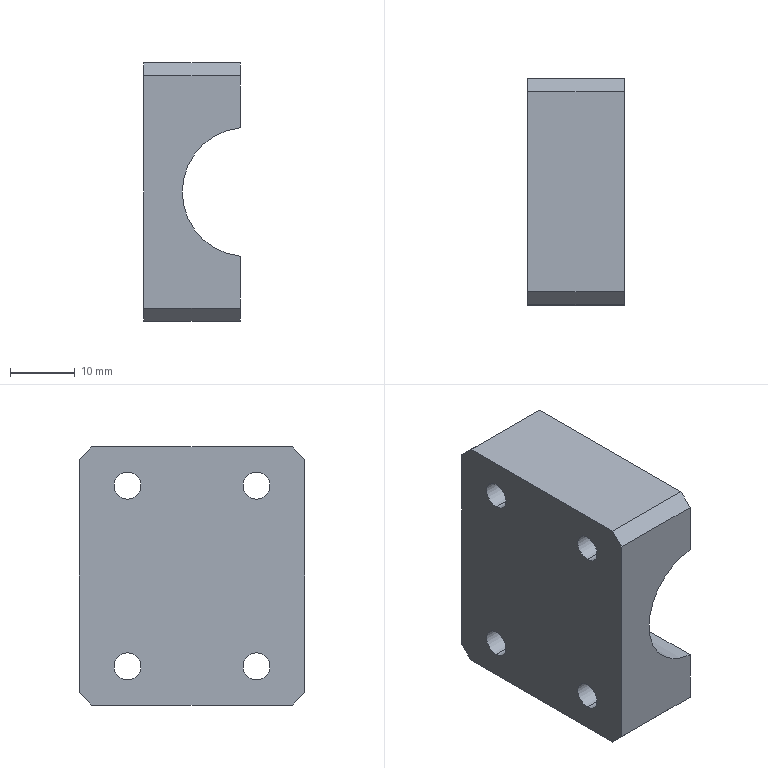Part | SolidWorks | features Chamfer 1, Extrusion 1, HoleWzd 1 | 1 solid | 20 faces | box 15 x 35 x 40 mm | volume 15250 mm3 | plane 11 | cylinder 9 | commonest cylinder face diameters 4.2 x8 20 x1
STEP:
#1=CARTESIAN_POINT('',(-7.5,10.,16.1));
#2=VERTEX_POINT('',#1);
#3=CARTESIAN_POINT('',(-7.5,10.,11.9));
#4=VERTEX_POINT('',#3);
#5=CARTESIAN_POINT('',(-7.5,10.,14.));
#6=DIRECTION('',(1.,0.,0.));
#7=DIRECTION('',(0.,0.,-1.));
#8=AXIS2_PLACEMENT_3D('',#5,#6,#7);
#9=CIRCLE('',#8,2.1);
#10=EDGE_CURVE('',#2,#4,#9,.T.);
#11=ORIENTED_EDGE('',*,*,#10,.F.);
#12=CARTESIAN_POINT('',(7.5,10.,16.1));
#13=VERTEX_POINT('',#12);
#14=CARTESIAN_POINT('',(7.5,10.,16.1));
#15=DIRECTION('',(1.,0.,0.));
#16=VECTOR('',#15,1000.);
#17=LINE('',#14,#16);
#18=EDGE_CURVE('',#2,#13,#17,.T.);
#19=ORIENTED_EDGE('',*,*,#18,.T.);
#20=CARTESIAN_POINT('',(7.5,10.,11.9));
#21=VERTEX_POINT('',#20);
#22=CARTESIAN_POINT('',(7.5,10.,14.));
#23=DIRECTION('',(1.,0.,0.));
#24=DIRECTION('',(0.,0.,-1.));
#25=AXIS2_PLACEMENT_3D('',#22,#23,#24);
#26=CIRCLE('',#25,2.1);
#27=EDGE_CURVE('',#13,#21,#26,.T.);
#28=ORIENTED_EDGE('',*,*,#27,.T.);
#29=CARTESIAN_POINT('',(7.5,10.,11.9));
#30=DIRECTION('',(1.,0.,0.));
#31=VECTOR('',#30,1000.);
#32=LINE('',#29,#31);
#33=EDGE_CURVE('',#4,#21,#32,.T.);
#34=ORIENTED_EDGE('',*,*,#33,.F.);
#35=EDGE_LOOP('',(#11,#19,#28,#34));
#36=FACE_OUTER_BOUND('',#35,.T.);
#37=CARTESIAN_POINT('',(7.5,10.,14.));
#38=DIRECTION('',(1.,0.,0.));
#39=DIRECTION('',(0.,0.,-1.));
#40=AXIS2_PLACEMENT_3D('',#37,#38,#39);
#41=CYLINDRICAL_SURFACE('',#40,2.1);
#42=ADVANCED_FACE('',(#36),#41,.F.);
#43=CARTESIAN_POINT('',(-7.5,10.,-11.9));
#44=VERTEX_POINT('',#43);
#45=CARTESIAN_POINT('',(-7.5,10.,-16.1));
#46=VERTEX_POINT('',#45);
#47=CARTESIAN_POINT('',(-7.5,10.,-14.));
#48=DIRECTION('',(1.,0.,0.));
#49=DIRECTION('',(0.,0.,-1.));
#50=AXIS2_PLACEMENT_3D('',#47,#48,#49);
#51=CIRCLE('',#50,2.1);
#52=EDGE_CURVE('',#44,#46,#51,.T.);
#53=ORIENTED_EDGE('',*,*,#52,.F.);
#54=CARTESIAN_POINT('',(7.5,10.,-11.9));
#55=VERTEX_POINT('',#54);
#56=CARTESIAN_POINT('',(7.5,10.,-11.9));
#57=DIRECTION('',(1.,0.,0.));
#58=VECTOR('',#57,1000.);
#59=LINE('',#56,#58);
#60=EDGE_CURVE('',#44,#55,#59,.T.);
#61=ORIENTED_EDGE('',*,*,#60,.T.);
#62=CARTESIAN_POINT('',(7.5,10.,-16.1));
#63=VERTEX_POINT('',#62);
#64=CARTESIAN_POINT('',(7.5,10.,-14.));
#65=DIRECTION('',(1.,0.,0.));
#66=DIRECTION('',(0.,0.,-1.));
#67=AXIS2_PLACEMENT_3D('',#64,#65,#66);
#68=CIRCLE('',#67,2.1);
#69=EDGE_CURVE('',#55,#63,#68,.T.);
#70=ORIENTED_EDGE('',*,*,#69,.T.);
#71=CARTESIAN_POINT('',(7.5,10.,-16.1));
#72=DIRECTION('',(1.,0.,0.));
#73=VECTOR('',#72,1000.);
#74=LINE('',#71,#73);
#75=EDGE_CURVE('',#46,#63,#74,.T.);
#76=ORIENTED_EDGE('',*,*,#75,.F.);
#77=EDGE_LOOP('',(#53,#61,#70,#76));
#78=FACE_OUTER_BOUND('',#77,.T.);
#79=CARTESIAN_POINT('',(7.5,10.,-14.));
#80=DIRECTION('',(1.,0.,0.));
#81=DIRECTION('',(0.,0.,-1.));
#82=AXIS2_PLACEMENT_3D('',#79,#80,#81);
#83=CYLINDRICAL_SURFACE('',#82,2.1);
#84=ADVANCED_FACE('',(#78),#83,.F.);
#85=CARTESIAN_POINT('',(-7.5,-10.,-11.9));
#86=VERTEX_POINT('',#85);
#87=CARTESIAN_POINT('',(-7.5,-10.,-16.1));
#88=VERTEX_POINT('',#87);
#89=CARTESIAN_POINT('',(-7.5,-10.,-14.));
#90=DIRECTION('',(1.,0.,0.));
#91=DIRECTION('',(0.,0.,-1.));
#92=AXIS2_PLACEMENT_3D('',#89,#90,#91);
#93=CIRCLE('',#92,2.1);
#94=EDGE_CURVE('',#86,#88,#93,.T.);
#95=ORIENTED_EDGE('',*,*,#94,.F.);
#96=CARTESIAN_POINT('',(7.5,-10.,-11.9));
#97=VERTEX_POINT('',#96);
#98=CARTESIAN_POINT('',(7.5,-10.,-11.9));
#99=DIRECTION('',(1.,0.,0.));
#100=VECTOR('',#99,1000.);
#101=LINE('',#98,#100);
#102=EDGE_CURVE('',#86,#97,#101,.T.);
#103=ORIENTED_EDGE('',*,*,#102,.T.);
#104=CARTESIAN_POINT('',(7.5,-10.,-16.1));
#105=VERTEX_POINT('',#104);
#106=CARTESIAN_POINT('',(7.5,-10.,-14.));
#107=DIRECTION('',(1.,0.,0.));
#108=DIRECTION('',(0.,0.,-1.));
#109=AXIS2_PLACEMENT_3D('',#106,#107,#108);
#110=CIRCLE('',#109,2.1);
#111=EDGE_CURVE('',#97,#105,#110,.T.);
#112=ORIENTED_EDGE('',*,*,#111,.T.);
#113=CARTESIAN_POINT('',(7.5,-10.,-16.1));
#114=DIRECTION('',(1.,0.,0.));
#115=VECTOR('',#114,1000.);
#116=LINE('',#113,#115);
#117=EDGE_CURVE('',#88,#105,#116,.T.);
#118=ORIENTED_EDGE('',*,*,#117,.F.);
#119=EDGE_LOOP('',(#95,#103,#112,#118));
#120=FACE_OUTER_BOUND('',#119,.T.);
#121=CARTESIAN_POINT('',(7.5,-10.,-14.));
#122=DIRECTION('',(1.,0.,0.));
#123=DIRECTION('',(0.,0.,-1.));
#124=AXIS2_PLACEMENT_3D('',#121,#122,#123);
#125=CYLINDRICAL_SURFACE('',#124,2.1);
#126=ADVANCED_FACE('',(#120),#125,.F.);
#127=CARTESIAN_POINT('',(-7.5,-10.,16.1));
#128=VERTEX_POINT('',#127);
#129=CARTESIAN_POINT('',(-7.5,-10.,11.9));
#130=VERTEX_POINT('',#129);
#131=CARTESIAN_POINT('',(-7.5,-10.,14.));
#132=DIRECTION('',(1.,0.,0.));
#133=DIRECTION('',(0.,0.,-1.));
#134=AXIS2_PLACEMENT_3D('',#131,#132,#133);
#135=CIRCLE('',#134,2.1);
#136=EDGE_CURVE('',#128,#130,#135,.T.);
#137=ORIENTED_EDGE('',*,*,#136,.F.);
#138=CARTESIAN_POINT('',(7.5,-10.,16.1));
#139=VERTEX_POINT('',#138);
#140=CARTESIAN_POINT('',(7.5,-10.,16.1));
#141=DIRECTION('',(1.,0.,0.));
#142=VECTOR('',#141,1000.);
#143=LINE('',#140,#142);
#144=EDGE_CURVE('',#128,#139,#143,.T.);
#145=ORIENTED_EDGE('',*,*,#144,.T.);
#146=CARTESIAN_POINT('',(7.5,-10.,11.9));
#147=VERTEX_POINT('',#146);
#148=CARTESIAN_POINT('',(7.5,-10.,14.));
#149=DIRECTION('',(1.,0.,0.));
#150=DIRECTION('',(0.,0.,-1.));
#151=AXIS2_PLACEMENT_3D('',#148,#149,#150);
#152=CIRCLE('',#151,2.1);
#153=EDGE_CURVE('',#139,#147,#152,.T.);
#154=ORIENTED_EDGE('',*,*,#153,.T.);
#155=CARTESIAN_POINT('',(7.5,-10.,11.9));
#156=DIRECTION('',(1.,0.,0.));
#157=VECTOR('',#156,1000.);
#158=LINE('',#155,#157);
#159=EDGE_CURVE('',#130,#147,#158,.T.);
#160=ORIENTED_EDGE('',*,*,#159,.F.);
#161=EDGE_LOOP('',(#137,#145,#154,#160));
#162=FACE_OUTER_BOUND('',#161,.T.);
#163=CARTESIAN_POINT('',(7.5,-10.,14.));
#164=DIRECTION('',(1.,0.,0.));
#165=DIRECTION('',(0.,0.,-1.));
#166=AXIS2_PLACEMENT_3D('',#163,#164,#165);
#167=CYLINDRICAL_SURFACE('',#166,2.1);
#168=ADVANCED_FACE('',(#162),#167,.F.);
#169=CARTESIAN_POINT('',(-7.5,15.5,-20.));
#170=VERTEX_POINT('',#169);
#171=CARTESIAN_POINT('',(-7.5,-15.5,-20.));
#172=VERTEX_POINT('',#171);
#173=CARTESIAN_POINT('',(-7.5,17.5,-20.));
#174=DIRECTION('',(0.,-1.,0.));
#175=VECTOR('',#174,1000.);
#176=LINE('',#173,#175);
#177=EDGE_CURVE('',#170,#172,#176,.T.);
#178=ORIENTED_EDGE('',*,*,#177,.F.);
#179=CARTESIAN_POINT('',(7.5,15.5,-20.));
#180=VERTEX_POINT('',#179);
#181=CARTESIAN_POINT('',(7.5,15.5,-20.));
#182=DIRECTION('',(1.,0.,0.));
#183=VECTOR('',#182,1000.);
#184=LINE('',#181,#183);
#185=EDGE_CURVE('',#170,#180,#184,.T.);
#186=ORIENTED_EDGE('',*,*,#185,.T.);
#187=CARTESIAN_POINT('',(7.5,-15.5,-20.));
#188=VERTEX_POINT('',#187);
#189=CARTESIAN_POINT('',(7.5,17.5,-20.));
#190=DIRECTION('',(0.,-1.,0.));
#191=VECTOR('',#190,1000.);
#192=LINE('',#189,#191);
#193=EDGE_CURVE('',#180,#188,#192,.T.);
#194=ORIENTED_EDGE('',*,*,#193,.T.);
#195=CARTESIAN_POINT('',(-7.5,-15.5,-20.));
#196=DIRECTION('',(-1.,0.,0.));
#197=VECTOR('',#196,1000.);
#198=LINE('',#195,#197);
#199=EDGE_CURVE('',#188,#172,#198,.T.);
#200=ORIENTED_EDGE('',*,*,#199,.T.);
#201=EDGE_LOOP('',(#178,#186,#194,#200));
#202=FACE_OUTER_BOUND('',#201,.T.);
#203=CARTESIAN_POINT('',(-7.5,17.5,-20.));
#204=DIRECTION('',(0.,0.,1.));
#205=DIRECTION('',(1.,0.,0.));
#206=AXIS2_PLACEMENT_3D('',#203,#204,#205);
#207=PLANE('',#206);
#208=ADVANCED_FACE('',(#202),#207,.F.);
#209=CARTESIAN_POINT('',(-7.5,10.,14.));
#210=DIRECTION('',(1.,0.,0.));
#211=DIRECTION('',(0.,0.,-1.));
#212=AXIS2_PLACEMENT_3D('',#209,#210,#211);
#213=CIRCLE('',#212,2.1);
#214=EDGE_CURVE('',#4,#2,#213,.T.);
#215=ORIENTED_EDGE('',*,*,#214,.T.);
#216=ORIENTED_EDGE('',*,*,#10,.T.);
#217=EDGE_LOOP('',(#215,#216));
#218=FACE_BOUND('',#217,.T.);
#219=CARTESIAN_POINT('',(-7.5,10.,-14.));
#220=DIRECTION('',(1.,0.,0.));
#221=DIRECTION('',(0.,0.,-1.));
#222=AXIS2_PLACEMENT_3D('',#219,#220,#221);
#223=CIRCLE('',#222,2.1);
#224=EDGE_CURVE('',#46,#44,#223,.T.);
#225=ORIENTED_EDGE('',*,*,#224,.T.);
#226=ORIENTED_EDGE('',*,*,#52,.T.);
#227=EDGE_LOOP('',(#225,#226));
#228=FACE_BOUND('',#227,.T.);
#229=CARTESIAN_POINT('',(-7.5,-10.,-14.));
#230=DIRECTION('',(1.,0.,0.));
#231=DIRECTION('',(0.,0.,-1.));
#232=AXIS2_PLACEMENT_3D('',#229,#230,#231);
#233=CIRCLE('',#232,2.1);
#234=EDGE_CURVE('',#88,#86,#233,.T.);
#235=ORIENTED_EDGE('',*,*,#234,.T.);
#236=ORIENTED_EDGE('',*,*,#94,.T.);
#237=EDGE_LOOP('',(#235,#236));
#238=FACE_BOUND('',#237,.T.);
#239=CARTESIAN_POINT('',(-7.5,-10.,14.));
#240=DIRECTION('',(1.,0.,0.));
#241=DIRECTION('',(0.,0.,-1.));
#242=AXIS2_PLACEMENT_3D('',#239,#240,#241);
#243=CIRCLE('',#242,2.1);
#244=EDGE_CURVE('',#130,#128,#243,.T.);
#245=ORIENTED_EDGE('',*,*,#244,.T.);
#246=ORIENTED_EDGE('',*,*,#136,.T.);
#247=EDGE_LOOP('',(#245,#246));
#248=FACE_BOUND('',#247,.T.);
#249=CARTESIAN_POINT('',(-7.5,-17.5,-18.));
#250=VERTEX_POINT('',#249);
#251=CARTESIAN_POINT('',(-7.5,-17.5,18.));
#252=VERTEX_POINT('',#251);
#253=CARTESIAN_POINT('',(-7.5,-17.5,20.));
#254=DIRECTION('',(0.,0.,1.));
#255=VECTOR('',#254,1000.);
#256=LINE('',#253,#255);
#257=EDGE_CURVE('',#250,#252,#256,.T.);
#258=ORIENTED_EDGE('',*,*,#257,.T.);
#259=CARTESIAN_POINT('',(-7.5,-15.5,20.));
#260=VERTEX_POINT('',#259);
#261=CARTESIAN_POINT('',(-7.5,-15.5,20.));
#262=DIRECTION('',(0.,0.7071,0.7071));
#263=VECTOR('',#262,1000.);
#264=LINE('',#261,#263);
#265=EDGE_CURVE('',#252,#260,#264,.T.);
#266=ORIENTED_EDGE('',*,*,#265,.T.);
#267=CARTESIAN_POINT('',(-7.5,15.5,20.));
#268=VERTEX_POINT('',#267);
#269=CARTESIAN_POINT('',(-7.5,17.5,20.));
#270=DIRECTION('',(0.,-1.,0.));
#271=VECTOR('',#270,1000.);
#272=LINE('',#269,#271);
#273=EDGE_CURVE('',#268,#260,#272,.T.);
#274=ORIENTED_EDGE('',*,*,#273,.F.);
#275=CARTESIAN_POINT('',(-7.5,17.5,18.));
#276=VERTEX_POINT('',#275);
#277=CARTESIAN_POINT('',(-7.5,17.5,18.));
#278=DIRECTION('',(0.,0.7071,-0.7071));
#279=VECTOR('',#278,1000.);
#280=LINE('',#277,#279);
#281=EDGE_CURVE('',#268,#276,#280,.T.);
#282=ORIENTED_EDGE('',*,*,#281,.T.);
#283=CARTESIAN_POINT('',(-7.5,17.5,-18.));
#284=VERTEX_POINT('',#283);
#285=CARTESIAN_POINT('',(-7.5,17.5,20.));
#286=DIRECTION('',(0.,0.,1.));
#287=VECTOR('',#286,1000.);
#288=LINE('',#285,#287);
#289=EDGE_CURVE('',#284,#276,#288,.T.);
#290=ORIENTED_EDGE('',*,*,#289,.F.);
#291=CARTESIAN_POINT('',(-7.5,17.5,-18.));
#292=DIRECTION('',(0.,-0.7071,-0.7071));
#293=VECTOR('',#292,1000.);
#294=LINE('',#291,#293);
#295=EDGE_CURVE('',#284,#170,#294,.T.);
#296=ORIENTED_EDGE('',*,*,#295,.T.);
#297=ORIENTED_EDGE('',*,*,#177,.T.);
#298=CARTESIAN_POINT('',(-7.5,-15.5,-20.));
#299=DIRECTION('',(0.,-0.7071,0.7071));
#300=VECTOR('',#299,1000.);
#301=LINE('',#298,#300);
#302=EDGE_CURVE('',#172,#250,#301,.T.);
#303=ORIENTED_EDGE('',*,*,#302,.T.);
#304=EDGE_LOOP('',(#258,#266,#274,#282,#290,#296,#297,#303));
#305=FACE_OUTER_BOUND('',#304,.T.);
#306=CARTESIAN_POINT('',(-7.5,17.5,20.));
#307=DIRECTION('',(1.,0.,0.));
#308=DIRECTION('',(0.,0.,-1.));
#309=AXIS2_PLACEMENT_3D('',#306,#307,#308);
#310=PLANE('',#309);
#311=ADVANCED_FACE('',(#218,#228,#238,#248,#305),#310,.F.);
#312=ORIENTED_EDGE('',*,*,#273,.T.);
#313=CARTESIAN_POINT('',(7.5,-15.5,20.));
#314=VERTEX_POINT('',#313);
#315=CARTESIAN_POINT('',(-7.5,-15.5,20.));
#316=DIRECTION('',(1.,0.,0.));
#317=VECTOR('',#316,1000.);
#318=LINE('',#315,#317);
#319=EDGE_CURVE('',#260,#314,#318,.T.);
#320=ORIENTED_EDGE('',*,*,#319,.T.);
#321=CARTESIAN_POINT('',(7.5,15.5,20.));
#322=VERTEX_POINT('',#321);
#323=CARTESIAN_POINT('',(7.5,17.5,20.));
#324=DIRECTION('',(0.,-1.,0.));
#325=VECTOR('',#324,1000.);
#326=LINE('',#323,#325);
#327=EDGE_CURVE('',#322,#314,#326,.T.);
#328=ORIENTED_EDGE('',*,*,#327,.F.);
#329=CARTESIAN_POINT('',(-7.5,15.5,20.));
#330=DIRECTION('',(-1.,0.,0.));
#331=VECTOR('',#330,1000.);
#332=LINE('',#329,#331);
#333=EDGE_CURVE('',#322,#268,#332,.T.);
#334=ORIENTED_EDGE('',*,*,#333,.T.);
#335=EDGE_LOOP('',(#312,#320,#328,#334));
#336=FACE_OUTER_BOUND('',#335,.T.);
#337=CARTESIAN_POINT('',(-7.5,17.5,20.));
#338=DIRECTION('',(0.,0.,-1.));
#339=DIRECTION('',(-1.,0.,0.));
#340=AXIS2_PLACEMENT_3D('',#337,#338,#339);
#341=PLANE('',#340);
#342=ADVANCED_FACE('',(#336),#341,.F.);
#343=CARTESIAN_POINT('',(7.5,10.,14.));
#344=DIRECTION('',(1.,0.,0.));
#345=DIRECTION('',(0.,0.,-1.));
#346=AXIS2_PLACEMENT_3D('',#343,#344,#345);
#347=CIRCLE('',#346,2.1);
#348=EDGE_CURVE('',#21,#13,#347,.T.);
#349=ORIENTED_EDGE('',*,*,#348,.F.);
#350=ORIENTED_EDGE('',*,*,#27,.F.);
#351=EDGE_LOOP('',(#349,#350));
#352=FACE_BOUND('',#351,.T.);
#353=CARTESIAN_POINT('',(7.5,-10.,14.));
#354=DIRECTION('',(1.,0.,0.));
#355=DIRECTION('',(0.,0.,-1.));
#356=AXIS2_PLACEMENT_3D('',#353,#354,#355);
#357=CIRCLE('',#356,2.1);
#358=EDGE_CURVE('',#147,#139,#357,.T.);
#359=ORIENTED_EDGE('',*,*,#358,.F.);
#360=ORIENTED_EDGE('',*,*,#153,.F.);
#361=EDGE_LOOP('',(#359,#360));
#362=FACE_BOUND('',#361,.T.);
#363=ORIENTED_EDGE('',*,*,#327,.T.);
#364=CARTESIAN_POINT('',(7.5,-17.5,18.));
#365=VERTEX_POINT('',#364);
#366=CARTESIAN_POINT('',(7.5,-15.5,20.));
#367=DIRECTION('',(0.,-0.7071,-0.7071));
#368=VECTOR('',#367,1000.);
#369=LINE('',#366,#368);
#370=EDGE_CURVE('',#314,#365,#369,.T.);
#371=ORIENTED_EDGE('',*,*,#370,.T.);
#372=CARTESIAN_POINT('',(7.5,-17.5,9.95));
#373=VERTEX_POINT('',#372);
#374=CARTESIAN_POINT('',(7.5,-17.5,20.));
#375=DIRECTION('',(0.,0.,-1.));
#376=VECTOR('',#375,1000.);
#377=LINE('',#374,#376);
#378=EDGE_CURVE('',#365,#373,#377,.T.);
#379=ORIENTED_EDGE('',*,*,#378,.T.);
#380=CARTESIAN_POINT('',(7.5,17.5,9.95));
#381=VERTEX_POINT('',#380);
#382=CARTESIAN_POINT('',(7.5,17.5,9.95));
#383=DIRECTION('',(0.,-1.,0.));
#384=VECTOR('',#383,1000.);
#385=LINE('',#382,#384);
#386=EDGE_CURVE('',#381,#373,#385,.T.);
#387=ORIENTED_EDGE('',*,*,#386,.F.);
#388=CARTESIAN_POINT('',(7.5,17.5,18.));
#389=VERTEX_POINT('',#388);
#390=CARTESIAN_POINT('',(7.5,17.5,20.));
#391=DIRECTION('',(0.,0.,-1.));
#392=VECTOR('',#391,1000.);
#393=LINE('',#390,#392);
#394=EDGE_CURVE('',#389,#381,#393,.T.);
#395=ORIENTED_EDGE('',*,*,#394,.F.);
#396=CARTESIAN_POINT('',(7.5,17.5,18.));
#397=DIRECTION('',(0.,-0.7071,0.7071));
#398=VECTOR('',#397,1000.);
#399=LINE('',#396,#398);
#400=EDGE_CURVE('',#389,#322,#399,.T.);
#401=ORIENTED_EDGE('',*,*,#400,.T.);
#402=EDGE_LOOP('',(#363,#371,#379,#387,#395,#401));
#403=FACE_OUTER_BOUND('',#402,.T.);
#404=CARTESIAN_POINT('',(7.5,17.5,20.));
#405=DIRECTION('',(-1.,0.,0.));
#406=DIRECTION('',(0.,0.,1.));
#407=AXIS2_PLACEMENT_3D('',#404,#405,#406);
#408=PLANE('',#407);
#409=ADVANCED_FACE('',(#352,#362,#403),#408,.F.);
#410=CARTESIAN_POINT('',(7.5,-17.5,-9.95));
#411=VERTEX_POINT('',#410);
#412=CARTESIAN_POINT('',(8.5,-17.5,0.));
#413=DIRECTION('',(0.,-1.,0.));
#414=DIRECTION('',(0.,0.,1.));
#415=AXIS2_PLACEMENT_3D('',#412,#413,#414);
#416=CIRCLE('',#415,10.);
#417=EDGE_CURVE('',#373,#411,#416,.T.);
#418=ORIENTED_EDGE('',*,*,#417,.T.);
#419=CARTESIAN_POINT('',(7.5,17.5,-9.95));
#420=VERTEX_POINT('',#419);
#421=CARTESIAN_POINT('',(7.5,17.5,-9.95));
#422=DIRECTION('',(0.,-1.,0.));
#423=VECTOR('',#422,1000.);
#424=LINE('',#421,#423);
#425=EDGE_CURVE('',#420,#411,#424,.T.);
#426=ORIENTED_EDGE('',*,*,#425,.F.);
#427=CARTESIAN_POINT('',(8.5,17.5,0.));
#428=DIRECTION('',(0.,-1.,0.));
#429=DIRECTION('',(0.,0.,1.));
#430=AXIS2_PLACEMENT_3D('',#427,#428,#429);
#431=CIRCLE('',#430,10.);
#432=EDGE_CURVE('',#381,#420,#431,.T.);
#433=ORIENTED_EDGE('',*,*,#432,.F.);
#434=ORIENTED_EDGE('',*,*,#386,.T.);
#435=EDGE_LOOP('',(#418,#426,#433,#434));
#436=FACE_OUTER_BOUND('',#435,.T.);
#437=CARTESIAN_POINT('',(8.5,17.5,0.));
#438=DIRECTION('',(0.,-1.,0.));
#439=DIRECTION('',(0.,0.,-1.));
#440=AXIS2_PLACEMENT_3D('',#437,#438,#439);
#441=CYLINDRICAL_SURFACE('',#440,10.);
#442=ADVANCED_FACE('',(#436),#441,.F.);
#443=CARTESIAN_POINT('',(7.5,10.,-14.));
#444=DIRECTION('',(1.,0.,0.));
#445=DIRECTION('',(0.,0.,-1.));
#446=AXIS2_PLACEMENT_3D('',#443,#444,#445);
#447=CIRCLE('',#446,2.1);
#448=EDGE_CURVE('',#63,#55,#447,.T.);
#449=ORIENTED_EDGE('',*,*,#448,.F.);
#450=ORIENTED_EDGE('',*,*,#69,.F.);
#451=EDGE_LOOP('',(#449,#450));
#452=FACE_BOUND('',#451,.T.);
#453=CARTESIAN_POINT('',(7.5,-10.,-14.));
#454=DIRECTION('',(1.,0.,0.));
#455=DIRECTION('',(0.,0.,-1.));
#456=AXIS2_PLACEMENT_3D('',#453,#454,#455);
#457=CIRCLE('',#456,2.1);
#458=EDGE_CURVE('',#105,#97,#457,.T.);
#459=ORIENTED_EDGE('',*,*,#458,.F.);
#460=ORIENTED_EDGE('',*,*,#111,.F.);
#461=EDGE_LOOP('',(#459,#460));
#462=FACE_BOUND('',#461,.T.);
#463=ORIENTED_EDGE('',*,*,#193,.F.);
#464=CARTESIAN_POINT('',(7.5,17.5,-18.));
#465=VERTEX_POINT('',#464);
#466=CARTESIAN_POINT('',(7.5,17.5,-18.));
#467=DIRECTION('',(0.,0.7071,0.7071));
#468=VECTOR('',#467,1000.);
#469=LINE('',#466,#468);
#470=EDGE_CURVE('',#180,#465,#469,.T.);
#471=ORIENTED_EDGE('',*,*,#470,.T.);
#472=CARTESIAN_POINT('',(7.5,17.5,-9.95));
#473=DIRECTION('',(0.,0.,-1.));
#474=VECTOR('',#473,1000.);
#475=LINE('',#472,#474);
#476=EDGE_CURVE('',#420,#465,#475,.T.);
#477=ORIENTED_EDGE('',*,*,#476,.F.);
#478=ORIENTED_EDGE('',*,*,#425,.T.);
#479=CARTESIAN_POINT('',(7.5,-17.5,-18.));
#480=VERTEX_POINT('',#479);
#481=CARTESIAN_POINT('',(7.5,-17.5,-9.95));
#482=DIRECTION('',(0.,0.,-1.));
#483=VECTOR('',#482,1000.);
#484=LINE('',#481,#483);
#485=EDGE_CURVE('',#411,#480,#484,.T.);
#486=ORIENTED_EDGE('',*,*,#485,.T.);
#487=CARTESIAN_POINT('',(7.5,-15.5,-20.));
#488=DIRECTION('',(0.,0.7071,-0.7071));
#489=VECTOR('',#488,1000.);
#490=LINE('',#487,#489);
#491=EDGE_CURVE('',#480,#188,#490,.T.);
#492=ORIENTED_EDGE('',*,*,#491,.T.);
#493=EDGE_LOOP('',(#463,#471,#477,#478,#486,#492));
#494=FACE_OUTER_BOUND('',#493,.T.);
#495=CARTESIAN_POINT('',(7.5,17.5,-9.95));
#496=DIRECTION('',(-1.,0.,0.));
#497=DIRECTION('',(0.,0.,1.));
#498=AXIS2_PLACEMENT_3D('',#495,#496,#497);
#499=PLANE('',#498);
#500=ADVANCED_FACE('',(#452,#462,#494),#499,.F.);
#501=ORIENTED_EDGE('',*,*,#289,.T.);
#502=CARTESIAN_POINT('',(7.5,17.5,18.));
#503=DIRECTION('',(1.,0.,0.));
#504=VECTOR('',#503,1000.);
#505=LINE('',#502,#504);
#506=EDGE_CURVE('',#276,#389,#505,.T.);
#507=ORIENTED_EDGE('',*,*,#506,.T.);
#508=ORIENTED_EDGE('',*,*,#394,.T.);
#509=ORIENTED_EDGE('',*,*,#432,.T.);
#510=ORIENTED_EDGE('',*,*,#476,.T.);
#511=CARTESIAN_POINT('',(-7.5,17.5,-18.));
#512=DIRECTION('',(-1.,0.,0.));
#513=VECTOR('',#512,1000.);
#514=LINE('',#511,#513);
#515=EDGE_CURVE('',#465,#284,#514,.T.);
#516=ORIENTED_EDGE('',*,*,#515,.T.);
#517=EDGE_LOOP('',(#501,#507,#508,#509,#510,#516));
#518=FACE_OUTER_BOUND('',#517,.T.);
#519=CARTESIAN_POINT('',(8.5,17.5,0.));
#520=DIRECTION('',(0.,1.,0.));
#521=DIRECTION('',(0.,0.,1.));
#522=AXIS2_PLACEMENT_3D('',#519,#520,#521);
#523=PLANE('',#522);
#524=ADVANCED_FACE('',(#518),#523,.T.);
#525=ORIENTED_EDGE('',*,*,#378,.F.);
#526=CARTESIAN_POINT('',(8.5,-17.5,18.));
#527=DIRECTION('',(-1.,0.,0.));
#528=VECTOR('',#527,1000.);
#529=LINE('',#526,#528);
#530=EDGE_CURVE('',#365,#252,#529,.T.);
#531=ORIENTED_EDGE('',*,*,#530,.T.);
#532=ORIENTED_EDGE('',*,*,#257,.F.);
#533=CARTESIAN_POINT('',(8.5,-17.5,-18.));
#534=DIRECTION('',(1.,0.,0.));
#535=VECTOR('',#534,1000.);
#536=LINE('',#533,#535);
#537=EDGE_CURVE('',#250,#480,#536,.T.);
#538=ORIENTED_EDGE('',*,*,#537,.T.);
#539=ORIENTED_EDGE('',*,*,#485,.F.);
#540=ORIENTED_EDGE('',*,*,#417,.F.);
#541=EDGE_LOOP('',(#525,#531,#532,#538,#539,#540));
#542=FACE_OUTER_BOUND('',#541,.T.);
#543=CARTESIAN_POINT('',(8.5,-17.5,0.));
#544=DIRECTION('',(0.,1.,0.));
#545=DIRECTION('',(0.,0.,1.));
#546=AXIS2_PLACEMENT_3D('',#543,#544,#545);
#547=PLANE('',#546);
#548=ADVANCED_FACE('',(#542),#547,.F.);
#549=ORIENTED_EDGE('',*,*,#265,.F.);
#550=ORIENTED_EDGE('',*,*,#530,.F.);
#551=ORIENTED_EDGE('',*,*,#370,.F.);
#552=ORIENTED_EDGE('',*,*,#319,.F.);
#553=EDGE_LOOP('',(#549,#550,#551,#552));
#554=FACE_OUTER_BOUND('',#553,.T.);
#555=CARTESIAN_POINT('',(-7.5,-15.5,20.));
#556=DIRECTION('',(0.,0.7071,-0.7071));
#557=DIRECTION('',(1.,0.,0.));
#558=AXIS2_PLACEMENT_3D('',#555,#556,#557);
#559=PLANE('',#558);
#560=ADVANCED_FACE('',(#554),#559,.F.);
#561=ORIENTED_EDGE('',*,*,#281,.F.);
#562=ORIENTED_EDGE('',*,*,#333,.F.);
#563=ORIENTED_EDGE('',*,*,#400,.F.);
#564=ORIENTED_EDGE('',*,*,#506,.F.);
#565=EDGE_LOOP('',(#561,#562,#563,#564));
#566=FACE_OUTER_BOUND('',#565,.T.);
#567=CARTESIAN_POINT('',(8.5,17.5,18.));
#568=DIRECTION('',(0.,0.7071,0.7071));
#569=DIRECTION('',(-1.,0.,0.));
#570=AXIS2_PLACEMENT_3D('',#567,#568,#569);
#571=PLANE('',#570);
#572=ADVANCED_FACE('',(#566),#571,.T.);
#573=ORIENTED_EDGE('',*,*,#470,.F.);
#574=ORIENTED_EDGE('',*,*,#185,.F.);
#575=ORIENTED_EDGE('',*,*,#295,.F.);
#576=ORIENTED_EDGE('',*,*,#515,.F.);
#577=EDGE_LOOP('',(#573,#574,#575,#576));
#578=FACE_OUTER_BOUND('',#577,.T.);
#579=CARTESIAN_POINT('',(8.5,17.5,-18.));
#580=DIRECTION('',(0.,0.7071,-0.7071));
#581=DIRECTION('',(1.,0.,0.));
#582=AXIS2_PLACEMENT_3D('',#579,#580,#581);
#583=PLANE('',#582);
#584=ADVANCED_FACE('',(#578),#583,.T.);
#585=ORIENTED_EDGE('',*,*,#491,.F.);
#586=ORIENTED_EDGE('',*,*,#537,.F.);
#587=ORIENTED_EDGE('',*,*,#302,.F.);
#588=ORIENTED_EDGE('',*,*,#199,.F.);
#589=EDGE_LOOP('',(#585,#586,#587,#588));
#590=FACE_OUTER_BOUND('',#589,.T.);
#591=CARTESIAN_POINT('',(-7.5,-15.5,-20.));
#592=DIRECTION('',(0.,0.7071,0.7071));
#593=DIRECTION('',(-1.,0.,0.));
#594=AXIS2_PLACEMENT_3D('',#591,#592,#593);
#595=PLANE('',#594);
#596=ADVANCED_FACE('',(#590),#595,.F.);
#597=ORIENTED_EDGE('',*,*,#144,.F.);
#598=ORIENTED_EDGE('',*,*,#244,.F.);
#599=ORIENTED_EDGE('',*,*,#159,.T.);
#600=ORIENTED_EDGE('',*,*,#358,.T.);
#601=EDGE_LOOP('',(#597,#598,#599,#600));
#602=FACE_OUTER_BOUND('',#601,.T.);
#603=CARTESIAN_POINT('',(7.5,-10.,14.));
#604=DIRECTION('',(1.,0.,0.));
#605=DIRECTION('',(0.,0.,-1.));
#606=AXIS2_PLACEMENT_3D('',#603,#604,#605);
#607=CYLINDRICAL_SURFACE('',#606,2.1);
#608=ADVANCED_FACE('',(#602),#607,.F.);
#609=ORIENTED_EDGE('',*,*,#102,.F.);
#610=ORIENTED_EDGE('',*,*,#234,.F.);
#611=ORIENTED_EDGE('',*,*,#117,.T.);
#612=ORIENTED_EDGE('',*,*,#458,.T.);
#613=EDGE_LOOP('',(#609,#610,#611,#612));
#614=FACE_OUTER_BOUND('',#613,.T.);
#615=CARTESIAN_POINT('',(7.5,-10.,-14.));
#616=DIRECTION('',(1.,0.,0.));
#617=DIRECTION('',(0.,0.,-1.));
#618=AXIS2_PLACEMENT_3D('',#615,#616,#617);
#619=CYLINDRICAL_SURFACE('',#618,2.1);
#620=ADVANCED_FACE('',(#614),#619,.F.);
#621=ORIENTED_EDGE('',*,*,#60,.F.);
#622=ORIENTED_EDGE('',*,*,#224,.F.);
#623=ORIENTED_EDGE('',*,*,#75,.T.);
#624=ORIENTED_EDGE('',*,*,#448,.T.);
#625=EDGE_LOOP('',(#621,#622,#623,#624));
#626=FACE_OUTER_BOUND('',#625,.T.);
#627=CARTESIAN_POINT('',(7.5,10.,-14.));
#628=DIRECTION('',(1.,0.,0.));
#629=DIRECTION('',(0.,0.,-1.));
#630=AXIS2_PLACEMENT_3D('',#627,#628,#629);
#631=CYLINDRICAL_SURFACE('',#630,2.1);
#632=ADVANCED_FACE('',(#626),#631,.F.);
#633=ORIENTED_EDGE('',*,*,#18,.F.);
#634=ORIENTED_EDGE('',*,*,#214,.F.);
#635=ORIENTED_EDGE('',*,*,#33,.T.);
#636=ORIENTED_EDGE('',*,*,#348,.T.);
#637=EDGE_LOOP('',(#633,#634,#635,#636));
#638=FACE_OUTER_BOUND('',#637,.T.);
#639=CARTESIAN_POINT('',(7.5,10.,14.));
#640=DIRECTION('',(1.,0.,0.));
#641=DIRECTION('',(0.,0.,-1.));
#642=AXIS2_PLACEMENT_3D('',#639,#640,#641);
#643=CYLINDRICAL_SURFACE('',#642,2.1);
#644=ADVANCED_FACE('',(#638),#643,.F.);
#645=CLOSED_SHELL('',(#42,#84,#126,#168,#208,#311,#342,#409,#442,#500,#524,#548,#560,#572,#584,#596,#608,#620,#632,#644));
#646=MANIFOLD_SOLID_BREP('',#645);
#647=CARTESIAN_POINT('',(0.,0.,0.));
#648=DIRECTION('',(0.,0.,1.));
#649=DIRECTION('',(1.,0.,0.));
#650=AXIS2_PLACEMENT_3D('',#647,#648,#649);
#651=(LENGTH_UNIT()NAMED_UNIT(*)SI_UNIT(.MILLI.,.METRE.));
#652=UNCERTAINTY_MEASURE_WITH_UNIT(LENGTH_MEASURE(0.00001),#651,'','');
#653=(NAMED_UNIT(*)PLANE_ANGLE_UNIT()SI_UNIT($,.RADIAN.));
#654=(NAMED_UNIT(*)SI_UNIT($,.STERADIAN.)SOLID_ANGLE_UNIT());
#655=(GEOMETRIC_REPRESENTATION_CONTEXT(3)GLOBAL_UNCERTAINTY_ASSIGNED_CONTEXT((#652))GLOBAL_UNIT_ASSIGNED_CONTEXT((#651,#653,#654))REPRESENTATION_CONTEXT('',''));
#656=ADVANCED_BREP_SHAPE_REPRESENTATION('',(#646,#650),#655);